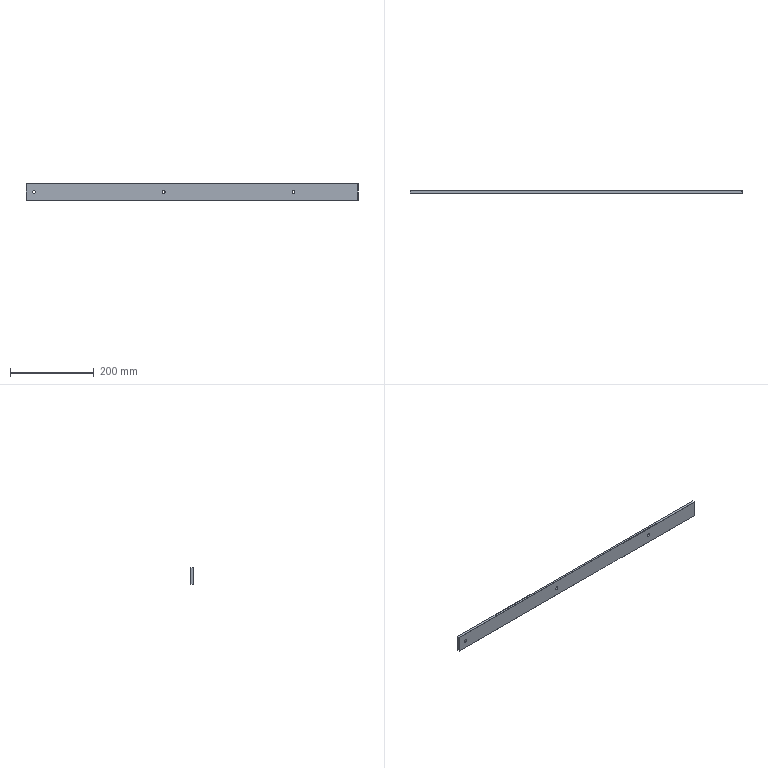Part | NX | 1 solid | 24 faces | box 793 x 6 x 40 mm | volume 189476 mm3 | plane 18 | cylinder 6 | commonest cylinder face diameters 7 x6
STEP:
#1=CARTESIAN_POINT('',(0.3,0.,-19.7));
#2=VERTEX_POINT('',#1);
#3=CARTESIAN_POINT('',(792.7,0.,-19.7));
#4=VERTEX_POINT('',#3);
#5=CARTESIAN_POINT('',(396.5,0.,-19.7));
#6=DIRECTION('',(1.,0.,0.));
#7=VECTOR('',#6,1000.);
#8=LINE('',#5,#7);
#9=EDGE_CURVE('',#2,#4,#8,.T.);
#10=ORIENTED_EDGE('',*,*,#9,.T.);
#11=CARTESIAN_POINT('',(792.7,0.,19.7));
#12=VERTEX_POINT('',#11);
#13=CARTESIAN_POINT('',(792.7,0.,0.));
#14=DIRECTION('',(0.,0.,1.));
#15=VECTOR('',#14,1000.);
#16=LINE('',#13,#15);
#17=EDGE_CURVE('',#4,#12,#16,.T.);
#18=ORIENTED_EDGE('',*,*,#17,.T.);
#19=CARTESIAN_POINT('',(0.3,0.,19.7));
#20=VERTEX_POINT('',#19);
#21=CARTESIAN_POINT('',(396.5,0.,19.7));
#22=DIRECTION('',(-1.,0.,0.));
#23=VECTOR('',#22,1000.);
#24=LINE('',#21,#23);
#25=EDGE_CURVE('',#12,#20,#24,.T.);
#26=ORIENTED_EDGE('',*,*,#25,.T.);
#27=CARTESIAN_POINT('',(0.3,0.,0.));
#28=DIRECTION('',(0.,0.,-1.));
#29=VECTOR('',#28,1000.);
#30=LINE('',#27,#29);
#31=EDGE_CURVE('',#20,#2,#30,.T.);
#32=ORIENTED_EDGE('',*,*,#31,.T.);
#33=EDGE_LOOP('',(#10,#18,#26,#32));
#34=FACE_BOUND('',#33,.T.);
#35=CARTESIAN_POINT('',(332.5,0.,0.));
#36=VERTEX_POINT('',#35);
#37=CARTESIAN_POINT('',(325.5,0.,0.));
#38=VERTEX_POINT('',#37);
#39=CARTESIAN_POINT('',(329.,0.,0.));
#40=DIRECTION('',(0.,-1.,0.));
#41=DIRECTION('',(-1.,0.,0.));
#42=AXIS2_PLACEMENT_3D('',#39,#40,#41);
#43=CIRCLE('',#42,3.5);
#44=EDGE_CURVE('',#36,#38,#43,.T.);
#45=ORIENTED_EDGE('',*,*,#44,.F.);
#46=CARTESIAN_POINT('',(329.,0.,0.));
#47=DIRECTION('',(0.,-1.,0.));
#48=DIRECTION('',(-1.,0.,0.));
#49=AXIS2_PLACEMENT_3D('',#46,#47,#48);
#50=CIRCLE('',#49,3.5);
#51=EDGE_CURVE('',#38,#36,#50,.T.);
#52=ORIENTED_EDGE('',*,*,#51,.F.);
#53=EDGE_LOOP('',(#45,#52));
#54=FACE_BOUND('',#53,.T.);
#55=CARTESIAN_POINT('',(642.5,0.,0.));
#56=VERTEX_POINT('',#55);
#57=CARTESIAN_POINT('',(635.5,0.,0.));
#58=VERTEX_POINT('',#57);
#59=CARTESIAN_POINT('',(639.,0.,0.));
#60=DIRECTION('',(0.,-1.,0.));
#61=DIRECTION('',(-1.,0.,0.));
#62=AXIS2_PLACEMENT_3D('',#59,#60,#61);
#63=CIRCLE('',#62,3.5);
#64=EDGE_CURVE('',#56,#58,#63,.T.);
#65=ORIENTED_EDGE('',*,*,#64,.F.);
#66=CARTESIAN_POINT('',(639.,0.,0.));
#67=DIRECTION('',(0.,-1.,0.));
#68=DIRECTION('',(-1.,0.,0.));
#69=AXIS2_PLACEMENT_3D('',#66,#67,#68);
#70=CIRCLE('',#69,3.5);
#71=EDGE_CURVE('',#58,#56,#70,.T.);
#72=ORIENTED_EDGE('',*,*,#71,.F.);
#73=EDGE_LOOP('',(#65,#72));
#74=FACE_BOUND('',#73,.T.);
#75=CARTESIAN_POINT('',(15.5,0.,0.));
#76=VERTEX_POINT('',#75);
#77=CARTESIAN_POINT('',(22.5,0.,0.));
#78=VERTEX_POINT('',#77);
#79=CARTESIAN_POINT('',(19.,0.,0.));
#80=DIRECTION('',(0.,-1.,0.));
#81=DIRECTION('',(-1.,0.,0.));
#82=AXIS2_PLACEMENT_3D('',#79,#80,#81);
#83=CIRCLE('',#82,3.5);
#84=EDGE_CURVE('',#76,#78,#83,.T.);
#85=ORIENTED_EDGE('',*,*,#84,.F.);
#86=CARTESIAN_POINT('',(19.,0.,0.));
#87=DIRECTION('',(0.,-1.,0.));
#88=DIRECTION('',(-1.,0.,0.));
#89=AXIS2_PLACEMENT_3D('',#86,#87,#88);
#90=CIRCLE('',#89,3.5);
#91=EDGE_CURVE('',#78,#76,#90,.T.);
#92=ORIENTED_EDGE('',*,*,#91,.F.);
#93=EDGE_LOOP('',(#85,#92));
#94=FACE_BOUND('',#93,.T.);
#95=CARTESIAN_POINT('',(0.,0.,0.));
#96=DIRECTION('',(0.,1.,0.));
#97=DIRECTION('',(1.,0.,0.));
#98=AXIS2_PLACEMENT_3D('',#95,#96,#97);
#99=PLANE('',#98);
#100=ADVANCED_FACE('',(#34,#54,#74,#94),#99,.F.);
#101=CARTESIAN_POINT('',(0.,5.7,-19.7));
#102=VERTEX_POINT('',#101);
#103=CARTESIAN_POINT('',(0.,0.3,-19.7));
#104=VERTEX_POINT('',#103);
#105=CARTESIAN_POINT('',(0.,3.,-19.7));
#106=DIRECTION('',(0.,-1.,0.));
#107=VECTOR('',#106,1000.);
#108=LINE('',#105,#107);
#109=EDGE_CURVE('',#102,#104,#108,.T.);
#110=ORIENTED_EDGE('',*,*,#109,.T.);
#111=CARTESIAN_POINT('',(0.,0.3,19.7));
#112=VERTEX_POINT('',#111);
#113=CARTESIAN_POINT('',(0.,0.3,0.));
#114=DIRECTION('',(0.,0.,-1.));
#115=VECTOR('',#114,1000.);
#116=LINE('',#113,#115);
#117=EDGE_CURVE('',#112,#104,#116,.T.);
#118=ORIENTED_EDGE('',*,*,#117,.F.);
#119=CARTESIAN_POINT('',(0.,5.7,19.7));
#120=VERTEX_POINT('',#119);
#121=CARTESIAN_POINT('',(0.,3.,19.7));
#122=DIRECTION('',(0.,-1.,0.));
#123=VECTOR('',#122,1000.);
#124=LINE('',#121,#123);
#125=EDGE_CURVE('',#120,#112,#124,.T.);
#126=ORIENTED_EDGE('',*,*,#125,.F.);
#127=CARTESIAN_POINT('',(0.,5.7,0.));
#128=DIRECTION('',(0.,0.,-1.));
#129=VECTOR('',#128,1000.);
#130=LINE('',#127,#129);
#131=EDGE_CURVE('',#120,#102,#130,.T.);
#132=ORIENTED_EDGE('',*,*,#131,.T.);
#133=EDGE_LOOP('',(#110,#118,#126,#132));
#134=FACE_BOUND('',#133,.T.);
#135=CARTESIAN_POINT('',(0.,0.,-20.));
#136=DIRECTION('',(-1.,0.,0.));
#137=DIRECTION('',(0.,0.,1.));
#138=AXIS2_PLACEMENT_3D('',#135,#136,#137);
#139=PLANE('',#138);
#140=ADVANCED_FACE('',(#134),#139,.T.);
#141=CARTESIAN_POINT('',(0.3,5.7,-20.));
#142=VERTEX_POINT('',#141);
#143=CARTESIAN_POINT('',(792.7,5.7,-20.));
#144=VERTEX_POINT('',#143);
#145=CARTESIAN_POINT('',(396.5,5.7,-20.));
#146=DIRECTION('',(1.,0.,0.));
#147=VECTOR('',#146,1000.);
#148=LINE('',#145,#147);
#149=EDGE_CURVE('',#142,#144,#148,.T.);
#150=ORIENTED_EDGE('',*,*,#149,.T.);
#151=CARTESIAN_POINT('',(792.7,0.3,-20.));
#152=VERTEX_POINT('',#151);
#153=CARTESIAN_POINT('',(792.7,3.,-20.));
#154=DIRECTION('',(0.,-1.,0.));
#155=VECTOR('',#154,1000.);
#156=LINE('',#153,#155);
#157=EDGE_CURVE('',#144,#152,#156,.T.);
#158=ORIENTED_EDGE('',*,*,#157,.T.);
#159=CARTESIAN_POINT('',(0.3,0.3,-20.));
#160=VERTEX_POINT('',#159);
#161=CARTESIAN_POINT('',(396.5,0.3,-20.));
#162=DIRECTION('',(1.,0.,0.));
#163=VECTOR('',#162,1000.);
#164=LINE('',#161,#163);
#165=EDGE_CURVE('',#160,#152,#164,.T.);
#166=ORIENTED_EDGE('',*,*,#165,.F.);
#167=CARTESIAN_POINT('',(0.3,3.,-20.));
#168=DIRECTION('',(0.,-1.,0.));
#169=VECTOR('',#168,1000.);
#170=LINE('',#167,#169);
#171=EDGE_CURVE('',#142,#160,#170,.T.);
#172=ORIENTED_EDGE('',*,*,#171,.F.);
#173=EDGE_LOOP('',(#150,#158,#166,#172));
#174=FACE_BOUND('',#173,.T.);
#175=CARTESIAN_POINT('',(793.,0.,-20.));
#176=DIRECTION('',(0.,0.,-1.));
#177=DIRECTION('',(0.,-1.,0.));
#178=AXIS2_PLACEMENT_3D('',#175,#176,#177);
#179=PLANE('',#178);
#180=ADVANCED_FACE('',(#174),#179,.T.);
#181=CARTESIAN_POINT('',(793.,5.7,-19.7));
#182=VERTEX_POINT('',#181);
#183=CARTESIAN_POINT('',(793.,5.7,19.7));
#184=VERTEX_POINT('',#183);
#185=CARTESIAN_POINT('',(793.,5.7,0.));
#186=DIRECTION('',(0.,0.,1.));
#187=VECTOR('',#186,1000.);
#188=LINE('',#185,#187);
#189=EDGE_CURVE('',#182,#184,#188,.T.);
#190=ORIENTED_EDGE('',*,*,#189,.T.);
#191=CARTESIAN_POINT('',(793.,0.3,19.7));
#192=VERTEX_POINT('',#191);
#193=CARTESIAN_POINT('',(793.,3.,19.7));
#194=DIRECTION('',(0.,-1.,0.));
#195=VECTOR('',#194,1000.);
#196=LINE('',#193,#195);
#197=EDGE_CURVE('',#184,#192,#196,.T.);
#198=ORIENTED_EDGE('',*,*,#197,.T.);
#199=CARTESIAN_POINT('',(793.,0.3,-19.7));
#200=VERTEX_POINT('',#199);
#201=CARTESIAN_POINT('',(793.,0.3,0.));
#202=DIRECTION('',(0.,0.,1.));
#203=VECTOR('',#202,1000.);
#204=LINE('',#201,#203);
#205=EDGE_CURVE('',#200,#192,#204,.T.);
#206=ORIENTED_EDGE('',*,*,#205,.F.);
#207=CARTESIAN_POINT('',(793.,3.,-19.7));
#208=DIRECTION('',(0.,-1.,0.));
#209=VECTOR('',#208,1000.);
#210=LINE('',#207,#209);
#211=EDGE_CURVE('',#182,#200,#210,.T.);
#212=ORIENTED_EDGE('',*,*,#211,.F.);
#213=EDGE_LOOP('',(#190,#198,#206,#212));
#214=FACE_BOUND('',#213,.T.);
#215=CARTESIAN_POINT('',(793.,0.,20.));
#216=DIRECTION('',(1.,0.,0.));
#217=DIRECTION('',(0.,1.,0.));
#218=AXIS2_PLACEMENT_3D('',#215,#216,#217);
#219=PLANE('',#218);
#220=ADVANCED_FACE('',(#214),#219,.T.);
#221=CARTESIAN_POINT('',(792.7,5.7,20.));
#222=VERTEX_POINT('',#221);
#223=CARTESIAN_POINT('',(0.3,5.7,20.));
#224=VERTEX_POINT('',#223);
#225=CARTESIAN_POINT('',(396.5,5.7,20.));
#226=DIRECTION('',(-1.,0.,0.));
#227=VECTOR('',#226,1000.);
#228=LINE('',#225,#227);
#229=EDGE_CURVE('',#222,#224,#228,.T.);
#230=ORIENTED_EDGE('',*,*,#229,.T.);
#231=CARTESIAN_POINT('',(0.3,0.3,20.));
#232=VERTEX_POINT('',#231);
#233=CARTESIAN_POINT('',(0.3,3.,20.));
#234=DIRECTION('',(0.,-1.,0.));
#235=VECTOR('',#234,1000.);
#236=LINE('',#233,#235);
#237=EDGE_CURVE('',#224,#232,#236,.T.);
#238=ORIENTED_EDGE('',*,*,#237,.T.);
#239=CARTESIAN_POINT('',(792.7,0.3,20.));
#240=VERTEX_POINT('',#239);
#241=CARTESIAN_POINT('',(396.5,0.3,20.));
#242=DIRECTION('',(-1.,0.,0.));
#243=VECTOR('',#242,1000.);
#244=LINE('',#241,#243);
#245=EDGE_CURVE('',#240,#232,#244,.T.);
#246=ORIENTED_EDGE('',*,*,#245,.F.);
#247=CARTESIAN_POINT('',(792.7,3.,20.));
#248=DIRECTION('',(0.,-1.,0.));
#249=VECTOR('',#248,1000.);
#250=LINE('',#247,#249);
#251=EDGE_CURVE('',#222,#240,#250,.T.);
#252=ORIENTED_EDGE('',*,*,#251,.F.);
#253=EDGE_LOOP('',(#230,#238,#246,#252));
#254=FACE_BOUND('',#253,.T.);
#255=CARTESIAN_POINT('',(0.,0.,20.));
#256=DIRECTION('',(0.,0.,1.));
#257=DIRECTION('',(1.,0.,0.));
#258=AXIS2_PLACEMENT_3D('',#255,#256,#257);
#259=PLANE('',#258);
#260=ADVANCED_FACE('',(#254),#259,.T.);
#261=CARTESIAN_POINT('',(0.3,6.,19.7));
#262=VERTEX_POINT('',#261);
#263=CARTESIAN_POINT('',(0.3,6.,-19.7));
#264=VERTEX_POINT('',#263);
#265=CARTESIAN_POINT('',(0.3,6.,0.));
#266=DIRECTION('',(0.,0.,-1.));
#267=VECTOR('',#266,1000.);
#268=LINE('',#265,#267);
#269=EDGE_CURVE('',#262,#264,#268,.T.);
#270=ORIENTED_EDGE('',*,*,#269,.F.);
#271=CARTESIAN_POINT('',(792.7,6.,19.7));
#272=VERTEX_POINT('',#271);
#273=CARTESIAN_POINT('',(396.5,6.,19.7));
#274=DIRECTION('',(-1.,0.,0.));
#275=VECTOR('',#274,1000.);
#276=LINE('',#273,#275);
#277=EDGE_CURVE('',#272,#262,#276,.T.);
#278=ORIENTED_EDGE('',*,*,#277,.F.);
#279=CARTESIAN_POINT('',(792.7,6.,-19.7));
#280=VERTEX_POINT('',#279);
#281=CARTESIAN_POINT('',(792.7,6.,0.));
#282=DIRECTION('',(0.,0.,1.));
#283=VECTOR('',#282,1000.);
#284=LINE('',#281,#283);
#285=EDGE_CURVE('',#280,#272,#284,.T.);
#286=ORIENTED_EDGE('',*,*,#285,.F.);
#287=CARTESIAN_POINT('',(396.5,6.,-19.7));
#288=DIRECTION('',(1.,0.,0.));
#289=VECTOR('',#288,1000.);
#290=LINE('',#287,#289);
#291=EDGE_CURVE('',#264,#280,#290,.T.);
#292=ORIENTED_EDGE('',*,*,#291,.F.);
#293=EDGE_LOOP('',(#270,#278,#286,#292));
#294=FACE_BOUND('',#293,.T.);
#295=CARTESIAN_POINT('',(332.5,6.,0.));
#296=VERTEX_POINT('',#295);
#297=CARTESIAN_POINT('',(325.5,6.,0.));
#298=VERTEX_POINT('',#297);
#299=CARTESIAN_POINT('',(329.,6.,0.));
#300=DIRECTION('',(0.,1.,0.));
#301=DIRECTION('',(1.,0.,0.));
#302=AXIS2_PLACEMENT_3D('',#299,#300,#301);
#303=CIRCLE('',#302,3.5);
#304=EDGE_CURVE('',#296,#298,#303,.T.);
#305=ORIENTED_EDGE('',*,*,#304,.F.);
#306=CARTESIAN_POINT('',(329.,6.,0.));
#307=DIRECTION('',(0.,1.,0.));
#308=DIRECTION('',(1.,0.,0.));
#309=AXIS2_PLACEMENT_3D('',#306,#307,#308);
#310=CIRCLE('',#309,3.5);
#311=EDGE_CURVE('',#298,#296,#310,.T.);
#312=ORIENTED_EDGE('',*,*,#311,.F.);
#313=EDGE_LOOP('',(#305,#312));
#314=FACE_BOUND('',#313,.T.);
#315=CARTESIAN_POINT('',(635.5,6.,0.));
#316=VERTEX_POINT('',#315);
#317=CARTESIAN_POINT('',(642.5,6.,0.));
#318=VERTEX_POINT('',#317);
#319=CARTESIAN_POINT('',(639.,6.,0.));
#320=DIRECTION('',(0.,1.,0.));
#321=DIRECTION('',(1.,0.,0.));
#322=AXIS2_PLACEMENT_3D('',#319,#320,#321);
#323=CIRCLE('',#322,3.5);
#324=EDGE_CURVE('',#316,#318,#323,.T.);
#325=ORIENTED_EDGE('',*,*,#324,.F.);
#326=CARTESIAN_POINT('',(639.,6.,0.));
#327=DIRECTION('',(0.,1.,0.));
#328=DIRECTION('',(1.,0.,0.));
#329=AXIS2_PLACEMENT_3D('',#326,#327,#328);
#330=CIRCLE('',#329,3.5);
#331=EDGE_CURVE('',#318,#316,#330,.T.);
#332=ORIENTED_EDGE('',*,*,#331,.F.);
#333=EDGE_LOOP('',(#325,#332));
#334=FACE_BOUND('',#333,.T.);
#335=CARTESIAN_POINT('',(22.5,6.,0.));
#336=VERTEX_POINT('',#335);
#337=CARTESIAN_POINT('',(15.5,6.,0.));
#338=VERTEX_POINT('',#337);
#339=CARTESIAN_POINT('',(19.,6.,0.));
#340=DIRECTION('',(0.,1.,0.));
#341=DIRECTION('',(1.,0.,0.));
#342=AXIS2_PLACEMENT_3D('',#339,#340,#341);
#343=CIRCLE('',#342,3.5);
#344=EDGE_CURVE('',#336,#338,#343,.T.);
#345=ORIENTED_EDGE('',*,*,#344,.F.);
#346=CARTESIAN_POINT('',(19.,6.,0.));
#347=DIRECTION('',(0.,1.,0.));
#348=DIRECTION('',(1.,0.,0.));
#349=AXIS2_PLACEMENT_3D('',#346,#347,#348);
#350=CIRCLE('',#349,3.5);
#351=EDGE_CURVE('',#338,#336,#350,.T.);
#352=ORIENTED_EDGE('',*,*,#351,.F.);
#353=EDGE_LOOP('',(#345,#352));
#354=FACE_BOUND('',#353,.T.);
#355=CARTESIAN_POINT('',(0.,6.,0.));
#356=DIRECTION('',(0.,1.,0.));
#357=DIRECTION('',(1.,0.,0.));
#358=AXIS2_PLACEMENT_3D('',#355,#356,#357);
#359=PLANE('',#358);
#360=ADVANCED_FACE('',(#294,#314,#334,#354),#359,.T.);
#361=ORIENTED_EDGE('',*,*,#84,.T.);
#362=CARTESIAN_POINT('',(22.5,6.,0.));
#363=DIRECTION('',(0.,-1.,0.));
#364=VECTOR('',#363,1000.);
#365=LINE('',#362,#364);
#366=EDGE_CURVE('',#336,#78,#365,.T.);
#367=ORIENTED_EDGE('',*,*,#366,.F.);
#368=ORIENTED_EDGE('',*,*,#344,.T.);
#369=CARTESIAN_POINT('',(15.5,6.,0.));
#370=DIRECTION('',(0.,-1.,0.));
#371=VECTOR('',#370,1000.);
#372=LINE('',#369,#371);
#373=EDGE_CURVE('',#338,#76,#372,.T.);
#374=ORIENTED_EDGE('',*,*,#373,.T.);
#375=EDGE_LOOP('',(#361,#367,#368,#374));
#376=FACE_BOUND('',#375,.T.);
#377=CARTESIAN_POINT('',(19.,6.,0.));
#378=DIRECTION('',(0.,-1.,0.));
#379=DIRECTION('',(1.,0.,0.));
#380=AXIS2_PLACEMENT_3D('',#377,#378,#379);
#381=CYLINDRICAL_SURFACE('',#380,3.5);
#382=ADVANCED_FACE('',(#376),#381,.F.);
#383=ORIENTED_EDGE('',*,*,#64,.T.);
#384=CARTESIAN_POINT('',(635.5,6.,0.));
#385=DIRECTION('',(0.,-1.,0.));
#386=VECTOR('',#385,1000.);
#387=LINE('',#384,#386);
#388=EDGE_CURVE('',#316,#58,#387,.T.);
#389=ORIENTED_EDGE('',*,*,#388,.F.);
#390=ORIENTED_EDGE('',*,*,#324,.T.);
#391=CARTESIAN_POINT('',(642.5,6.,0.));
#392=DIRECTION('',(0.,-1.,0.));
#393=VECTOR('',#392,1000.);
#394=LINE('',#391,#393);
#395=EDGE_CURVE('',#318,#56,#394,.T.);
#396=ORIENTED_EDGE('',*,*,#395,.T.);
#397=EDGE_LOOP('',(#383,#389,#390,#396));
#398=FACE_BOUND('',#397,.T.);
#399=CARTESIAN_POINT('',(639.,6.,0.));
#400=DIRECTION('',(0.,-1.,0.));
#401=DIRECTION('',(1.,0.,0.));
#402=AXIS2_PLACEMENT_3D('',#399,#400,#401);
#403=CYLINDRICAL_SURFACE('',#402,3.5);
#404=ADVANCED_FACE('',(#398),#403,.F.);
#405=ORIENTED_EDGE('',*,*,#304,.T.);
#406=CARTESIAN_POINT('',(325.5,6.,0.));
#407=DIRECTION('',(0.,-1.,0.));
#408=VECTOR('',#407,1000.);
#409=LINE('',#406,#408);
#410=EDGE_CURVE('',#38,#298,#409,.F.);
#411=ORIENTED_EDGE('',*,*,#410,.F.);
#412=ORIENTED_EDGE('',*,*,#51,.T.);
#413=CARTESIAN_POINT('',(332.5,6.,0.));
#414=DIRECTION('',(0.,-1.,0.));
#415=VECTOR('',#414,1000.);
#416=LINE('',#413,#415);
#417=EDGE_CURVE('',#36,#296,#416,.F.);
#418=ORIENTED_EDGE('',*,*,#417,.T.);
#419=EDGE_LOOP('',(#405,#411,#412,#418));
#420=FACE_BOUND('',#419,.T.);
#421=CARTESIAN_POINT('',(329.,6.,0.));
#422=DIRECTION('',(0.,-1.,0.));
#423=DIRECTION('',(1.,0.,0.));
#424=AXIS2_PLACEMENT_3D('',#421,#422,#423);
#425=CYLINDRICAL_SURFACE('',#424,3.5);
#426=ADVANCED_FACE('',(#420),#425,.F.);
#427=ORIENTED_EDGE('',*,*,#131,.F.);
#428=CARTESIAN_POINT('',(0.15,5.85,19.85));
#429=VERTEX_POINT('',#428);
#430=CARTESIAN_POINT('',(0.,5.7,19.7));
#431=DIRECTION('',(-0.5774,-0.5774,-0.5774));
#432=VECTOR('',#431,1000.);
#433=LINE('',#430,#432);
#434=EDGE_CURVE('',#429,#120,#433,.T.);
#435=ORIENTED_EDGE('',*,*,#434,.F.);
#436=CARTESIAN_POINT('',(20.,25.7,0.));
#437=DIRECTION('',(0.5774,0.5774,-0.5774));
#438=VECTOR('',#437,1000.);
#439=LINE('',#436,#438);
#440=EDGE_CURVE('',#429,#262,#439,.T.);
#441=ORIENTED_EDGE('',*,*,#440,.T.);
#442=ORIENTED_EDGE('',*,*,#269,.T.);
#443=CARTESIAN_POINT('',(0.15,5.85,-19.85));
#444=VERTEX_POINT('',#443);
#445=CARTESIAN_POINT('',(20.,25.7,0.));
#446=DIRECTION('',(-0.5774,-0.5774,-0.5774));
#447=VECTOR('',#446,1000.);
#448=LINE('',#445,#447);
#449=EDGE_CURVE('',#264,#444,#448,.T.);
#450=ORIENTED_EDGE('',*,*,#449,.T.);
#451=CARTESIAN_POINT('',(-19.7,-14.,0.));
#452=DIRECTION('',(-0.5774,-0.5774,0.5774));
#453=VECTOR('',#452,1000.);
#454=LINE('',#451,#453);
#455=EDGE_CURVE('',#444,#102,#454,.T.);
#456=ORIENTED_EDGE('',*,*,#455,.T.);
#457=EDGE_LOOP('',(#427,#435,#441,#442,#450,#456));
#458=FACE_BOUND('',#457,.T.);
#459=CARTESIAN_POINT('',(0.15,5.85,0.));
#460=DIRECTION('',(-0.7071,0.7071,0.));
#461=DIRECTION('',(0.,0.,1.));
#462=AXIS2_PLACEMENT_3D('',#459,#460,#461);
#463=PLANE('',#462);
#464=ADVANCED_FACE('',(#458),#463,.T.);
#465=ORIENTED_EDGE('',*,*,#31,.F.);
#466=CARTESIAN_POINT('',(0.15,0.15,19.85));
#467=VERTEX_POINT('',#466);
#468=CARTESIAN_POINT('',(20.,-19.7,0.));
#469=DIRECTION('',(-0.5774,0.5774,0.5774));
#470=VECTOR('',#469,1000.);
#471=LINE('',#468,#470);
#472=EDGE_CURVE('',#20,#467,#471,.T.);
#473=ORIENTED_EDGE('',*,*,#472,.T.);
#474=CARTESIAN_POINT('',(0.3,0.,20.));
#475=DIRECTION('',(0.5774,-0.5774,0.5774));
#476=VECTOR('',#475,1000.);
#477=LINE('',#474,#476);
#478=EDGE_CURVE('',#112,#467,#477,.T.);
#479=ORIENTED_EDGE('',*,*,#478,.F.);
#480=ORIENTED_EDGE('',*,*,#117,.T.);
#481=CARTESIAN_POINT('',(0.15,0.15,-19.85));
#482=VERTEX_POINT('',#481);
#483=CARTESIAN_POINT('',(-19.7,20.,0.));
#484=DIRECTION('',(0.5774,-0.5774,-0.5774));
#485=VECTOR('',#484,1000.);
#486=LINE('',#483,#485);
#487=EDGE_CURVE('',#104,#482,#486,.T.);
#488=ORIENTED_EDGE('',*,*,#487,.T.);
#489=CARTESIAN_POINT('',(20.,-19.7,0.));
#490=DIRECTION('',(0.5774,-0.5774,0.5774));
#491=VECTOR('',#490,1000.);
#492=LINE('',#489,#491);
#493=EDGE_CURVE('',#482,#2,#492,.T.);
#494=ORIENTED_EDGE('',*,*,#493,.T.);
#495=EDGE_LOOP('',(#465,#473,#479,#480,#488,#494));
#496=FACE_BOUND('',#495,.T.);
#497=CARTESIAN_POINT('',(0.15,0.15,0.));
#498=DIRECTION('',(-0.7071,-0.7071,0.));
#499=DIRECTION('',(-0.7071,0.7071,0.));
#500=AXIS2_PLACEMENT_3D('',#497,#498,#499);
#501=PLANE('',#500);
#502=ADVANCED_FACE('',(#496),#501,.T.);
#503=ORIENTED_EDGE('',*,*,#125,.T.);
#504=ORIENTED_EDGE('',*,*,#478,.T.);
#505=CARTESIAN_POINT('',(0.,0.,19.7));
#506=DIRECTION('',(-0.5774,-0.5774,-0.5774));
#507=VECTOR('',#506,1000.);
#508=LINE('',#505,#507);
#509=EDGE_CURVE('',#232,#467,#508,.T.);
#510=ORIENTED_EDGE('',*,*,#509,.F.);
#511=ORIENTED_EDGE('',*,*,#237,.F.);
#512=CARTESIAN_POINT('',(0.,6.,19.7));
#513=DIRECTION('',(0.5774,-0.5774,0.5774));
#514=VECTOR('',#513,1000.);
#515=LINE('',#512,#514);
#516=EDGE_CURVE('',#429,#224,#515,.T.);
#517=ORIENTED_EDGE('',*,*,#516,.F.);
#518=ORIENTED_EDGE('',*,*,#434,.T.);
#519=EDGE_LOOP('',(#503,#504,#510,#511,#517,#518));
#520=FACE_BOUND('',#519,.T.);
#521=CARTESIAN_POINT('',(0.15,3.,19.85));
#522=DIRECTION('',(0.7071,0.,-0.7071));
#523=DIRECTION('',(0.,-1.,0.));
#524=AXIS2_PLACEMENT_3D('',#521,#522,#523);
#525=PLANE('',#524);
#526=ADVANCED_FACE('',(#520),#525,.F.);
#527=ORIENTED_EDGE('',*,*,#229,.F.);
#528=CARTESIAN_POINT('',(792.85,5.85,19.85));
#529=VERTEX_POINT('',#528);
#530=CARTESIAN_POINT('',(812.7,25.7,0.));
#531=DIRECTION('',(0.5774,0.5774,-0.5774));
#532=VECTOR('',#531,1000.);
#533=LINE('',#530,#532);
#534=EDGE_CURVE('',#222,#529,#533,.T.);
#535=ORIENTED_EDGE('',*,*,#534,.T.);
#536=CARTESIAN_POINT('',(773.,25.7,0.));
#537=DIRECTION('',(-0.5774,0.5774,-0.5774));
#538=VECTOR('',#537,1000.);
#539=LINE('',#536,#538);
#540=EDGE_CURVE('',#529,#272,#539,.T.);
#541=ORIENTED_EDGE('',*,*,#540,.T.);
#542=ORIENTED_EDGE('',*,*,#277,.T.);
#543=ORIENTED_EDGE('',*,*,#440,.F.);
#544=ORIENTED_EDGE('',*,*,#516,.T.);
#545=EDGE_LOOP('',(#527,#535,#541,#542,#543,#544));
#546=FACE_BOUND('',#545,.T.);
#547=CARTESIAN_POINT('',(396.5,5.85,19.85));
#548=DIRECTION('',(0.,0.7071,0.7071));
#549=DIRECTION('',(1.,0.,0.));
#550=AXIS2_PLACEMENT_3D('',#547,#548,#549);
#551=PLANE('',#550);
#552=ADVANCED_FACE('',(#546),#551,.T.);
#553=ORIENTED_EDGE('',*,*,#25,.F.);
#554=CARTESIAN_POINT('',(792.85,0.15,19.85));
#555=VERTEX_POINT('',#554);
#556=CARTESIAN_POINT('',(773.,-19.7,0.));
#557=DIRECTION('',(0.5774,0.5774,0.5774));
#558=VECTOR('',#557,1000.);
#559=LINE('',#556,#558);
#560=EDGE_CURVE('',#12,#555,#559,.T.);
#561=ORIENTED_EDGE('',*,*,#560,.T.);
#562=CARTESIAN_POINT('',(812.7,-19.7,0.));
#563=DIRECTION('',(-0.5774,0.5774,0.5774));
#564=VECTOR('',#563,1000.);
#565=LINE('',#562,#564);
#566=EDGE_CURVE('',#555,#240,#565,.T.);
#567=ORIENTED_EDGE('',*,*,#566,.T.);
#568=ORIENTED_EDGE('',*,*,#245,.T.);
#569=ORIENTED_EDGE('',*,*,#509,.T.);
#570=ORIENTED_EDGE('',*,*,#472,.F.);
#571=EDGE_LOOP('',(#553,#561,#567,#568,#569,#570));
#572=FACE_BOUND('',#571,.T.);
#573=CARTESIAN_POINT('',(396.5,0.15,19.85));
#574=DIRECTION('',(0.,-0.7071,0.7071));
#575=DIRECTION('',(-1.,0.,0.));
#576=AXIS2_PLACEMENT_3D('',#573,#574,#575);
#577=PLANE('',#576);
#578=ADVANCED_FACE('',(#572),#577,.T.);
#579=ORIENTED_EDGE('',*,*,#197,.F.);
#580=CARTESIAN_POINT('',(812.7,-14.,0.));
#581=DIRECTION('',(-0.5774,0.5774,0.5774));
#582=VECTOR('',#581,1000.);
#583=LINE('',#580,#582);
#584=EDGE_CURVE('',#184,#529,#583,.T.);
#585=ORIENTED_EDGE('',*,*,#584,.T.);
#586=ORIENTED_EDGE('',*,*,#534,.F.);
#587=ORIENTED_EDGE('',*,*,#251,.T.);
#588=ORIENTED_EDGE('',*,*,#566,.F.);
#589=CARTESIAN_POINT('',(812.7,20.,0.));
#590=DIRECTION('',(0.5774,0.5774,-0.5774));
#591=VECTOR('',#590,1000.);
#592=LINE('',#589,#591);
#593=EDGE_CURVE('',#555,#192,#592,.T.);
#594=ORIENTED_EDGE('',*,*,#593,.T.);
#595=EDGE_LOOP('',(#579,#585,#586,#587,#588,#594));
#596=FACE_BOUND('',#595,.T.);
#597=CARTESIAN_POINT('',(792.85,3.,19.85));
#598=DIRECTION('',(0.7071,0.,0.7071));
#599=DIRECTION('',(0.,-1.,0.));
#600=AXIS2_PLACEMENT_3D('',#597,#598,#599);
#601=PLANE('',#600);
#602=ADVANCED_FACE('',(#596),#601,.T.);
#603=ORIENTED_EDGE('',*,*,#189,.F.);
#604=CARTESIAN_POINT('',(792.85,5.85,-19.85));
#605=VERTEX_POINT('',#604);
#606=CARTESIAN_POINT('',(798.7,0.,-14.));
#607=DIRECTION('',(-0.5774,0.5774,-0.5774));
#608=VECTOR('',#607,1000.);
#609=LINE('',#606,#608);
#610=EDGE_CURVE('',#182,#605,#609,.T.);
#611=ORIENTED_EDGE('',*,*,#610,.T.);
#612=CARTESIAN_POINT('',(773.,25.7,0.));
#613=DIRECTION('',(-0.5774,0.5774,0.5774));
#614=VECTOR('',#613,1000.);
#615=LINE('',#612,#614);
#616=EDGE_CURVE('',#605,#280,#615,.T.);
#617=ORIENTED_EDGE('',*,*,#616,.T.);
#618=ORIENTED_EDGE('',*,*,#285,.T.);
#619=ORIENTED_EDGE('',*,*,#540,.F.);
#620=ORIENTED_EDGE('',*,*,#584,.F.);
#621=EDGE_LOOP('',(#603,#611,#617,#618,#619,#620));
#622=FACE_BOUND('',#621,.T.);
#623=CARTESIAN_POINT('',(792.85,5.85,0.));
#624=DIRECTION('',(0.7071,0.7071,0.));
#625=DIRECTION('',(0.,0.,-1.));
#626=AXIS2_PLACEMENT_3D('',#623,#624,#625);
#627=PLANE('',#626);
#628=ADVANCED_FACE('',(#622),#627,.T.);
#629=ORIENTED_EDGE('',*,*,#17,.F.);
#630=CARTESIAN_POINT('',(792.85,0.15,-19.85));
#631=VERTEX_POINT('',#630);
#632=CARTESIAN_POINT('',(773.,-19.7,0.));
#633=DIRECTION('',(0.5774,0.5774,-0.5774));
#634=VECTOR('',#633,1000.);
#635=LINE('',#632,#634);
#636=EDGE_CURVE('',#4,#631,#635,.T.);
#637=ORIENTED_EDGE('',*,*,#636,.T.);
#638=CARTESIAN_POINT('',(792.7,0.,-20.));
#639=DIRECTION('',(0.5774,0.5774,0.5774));
#640=VECTOR('',#639,1000.);
#641=LINE('',#638,#640);
#642=EDGE_CURVE('',#631,#200,#641,.T.);
#643=ORIENTED_EDGE('',*,*,#642,.T.);
#644=ORIENTED_EDGE('',*,*,#205,.T.);
#645=ORIENTED_EDGE('',*,*,#593,.F.);
#646=ORIENTED_EDGE('',*,*,#560,.F.);
#647=EDGE_LOOP('',(#629,#637,#643,#644,#645,#646));
#648=FACE_BOUND('',#647,.T.);
#649=CARTESIAN_POINT('',(792.85,0.15,0.));
#650=DIRECTION('',(0.7071,-0.7071,0.));
#651=DIRECTION('',(0.,0.,-1.));
#652=AXIS2_PLACEMENT_3D('',#649,#650,#651);
#653=PLANE('',#652);
#654=ADVANCED_FACE('',(#648),#653,.T.);
#655=ORIENTED_EDGE('',*,*,#157,.F.);
#656=CARTESIAN_POINT('',(812.7,25.7,0.));
#657=DIRECTION('',(0.5774,0.5774,0.5774));
#658=VECTOR('',#657,1000.);
#659=LINE('',#656,#658);
#660=EDGE_CURVE('',#144,#605,#659,.T.);
#661=ORIENTED_EDGE('',*,*,#660,.T.);
#662=ORIENTED_EDGE('',*,*,#610,.F.);
#663=ORIENTED_EDGE('',*,*,#211,.T.);
#664=ORIENTED_EDGE('',*,*,#642,.F.);
#665=CARTESIAN_POINT('',(812.7,-19.7,0.));
#666=DIRECTION('',(-0.5774,0.5774,-0.5774));
#667=VECTOR('',#666,1000.);
#668=LINE('',#665,#667);
#669=EDGE_CURVE('',#631,#152,#668,.T.);
#670=ORIENTED_EDGE('',*,*,#669,.T.);
#671=EDGE_LOOP('',(#655,#661,#662,#663,#664,#670));
#672=FACE_BOUND('',#671,.T.);
#673=CARTESIAN_POINT('',(792.85,3.,-19.85));
#674=DIRECTION('',(0.7071,0.,-0.7071));
#675=DIRECTION('',(0.,-1.,0.));
#676=AXIS2_PLACEMENT_3D('',#673,#674,#675);
#677=PLANE('',#676);
#678=ADVANCED_FACE('',(#672),#677,.T.);
#679=ORIENTED_EDGE('',*,*,#9,.F.);
#680=ORIENTED_EDGE('',*,*,#493,.F.);
#681=CARTESIAN_POINT('',(-19.7,-19.7,0.));
#682=DIRECTION('',(0.5774,0.5774,-0.5774));
#683=VECTOR('',#682,1000.);
#684=LINE('',#681,#683);
#685=EDGE_CURVE('',#482,#160,#684,.T.);
#686=ORIENTED_EDGE('',*,*,#685,.T.);
#687=ORIENTED_EDGE('',*,*,#165,.T.);
#688=ORIENTED_EDGE('',*,*,#669,.F.);
#689=ORIENTED_EDGE('',*,*,#636,.F.);
#690=EDGE_LOOP('',(#679,#680,#686,#687,#688,#689));
#691=FACE_BOUND('',#690,.T.);
#692=CARTESIAN_POINT('',(396.5,0.15,-19.85));
#693=DIRECTION('',(0.,-0.7071,-0.7071));
#694=DIRECTION('',(0.,0.7071,-0.7071));
#695=AXIS2_PLACEMENT_3D('',#692,#693,#694);
#696=PLANE('',#695);
#697=ADVANCED_FACE('',(#691),#696,.T.);
#698=ORIENTED_EDGE('',*,*,#149,.F.);
#699=CARTESIAN_POINT('',(-19.7,25.7,0.));
#700=DIRECTION('',(-0.5774,0.5774,0.5774));
#701=VECTOR('',#700,1000.);
#702=LINE('',#699,#701);
#703=EDGE_CURVE('',#142,#444,#702,.T.);
#704=ORIENTED_EDGE('',*,*,#703,.T.);
#705=ORIENTED_EDGE('',*,*,#449,.F.);
#706=ORIENTED_EDGE('',*,*,#291,.T.);
#707=ORIENTED_EDGE('',*,*,#616,.F.);
#708=ORIENTED_EDGE('',*,*,#660,.F.);
#709=EDGE_LOOP('',(#698,#704,#705,#706,#707,#708));
#710=FACE_BOUND('',#709,.T.);
#711=CARTESIAN_POINT('',(396.5,5.85,-19.85));
#712=DIRECTION('',(0.,0.7071,-0.7071));
#713=DIRECTION('',(-1.,0.,0.));
#714=AXIS2_PLACEMENT_3D('',#711,#712,#713);
#715=PLANE('',#714);
#716=ADVANCED_FACE('',(#710),#715,.T.);
#717=ORIENTED_EDGE('',*,*,#109,.F.);
#718=ORIENTED_EDGE('',*,*,#455,.F.);
#719=ORIENTED_EDGE('',*,*,#703,.F.);
#720=ORIENTED_EDGE('',*,*,#171,.T.);
#721=ORIENTED_EDGE('',*,*,#685,.F.);
#722=ORIENTED_EDGE('',*,*,#487,.F.);
#723=EDGE_LOOP('',(#717,#718,#719,#720,#721,#722));
#724=FACE_BOUND('',#723,.T.);
#725=CARTESIAN_POINT('',(0.15,3.,-19.85));
#726=DIRECTION('',(-0.7071,0.,-0.7071));
#727=DIRECTION('',(-0.7071,0.,0.7071));
#728=AXIS2_PLACEMENT_3D('',#725,#726,#727);
#729=PLANE('',#728);
#730=ADVANCED_FACE('',(#724),#729,.T.);
#731=ORIENTED_EDGE('',*,*,#44,.T.);
#732=ORIENTED_EDGE('',*,*,#410,.T.);
#733=ORIENTED_EDGE('',*,*,#311,.T.);
#734=ORIENTED_EDGE('',*,*,#417,.F.);
#735=EDGE_LOOP('',(#731,#732,#733,#734));
#736=FACE_BOUND('',#735,.T.);
#737=CARTESIAN_POINT('',(329.,6.,0.));
#738=DIRECTION('',(0.,-1.,0.));
#739=DIRECTION('',(1.,0.,0.));
#740=AXIS2_PLACEMENT_3D('',#737,#738,#739);
#741=CYLINDRICAL_SURFACE('',#740,3.5);
#742=ADVANCED_FACE('',(#736),#741,.F.);
#743=ORIENTED_EDGE('',*,*,#366,.T.);
#744=ORIENTED_EDGE('',*,*,#91,.T.);
#745=ORIENTED_EDGE('',*,*,#373,.F.);
#746=ORIENTED_EDGE('',*,*,#351,.T.);
#747=EDGE_LOOP('',(#743,#744,#745,#746));
#748=FACE_BOUND('',#747,.T.);
#749=CARTESIAN_POINT('',(19.,6.,0.));
#750=DIRECTION('',(0.,-1.,0.));
#751=DIRECTION('',(1.,0.,0.));
#752=AXIS2_PLACEMENT_3D('',#749,#750,#751);
#753=CYLINDRICAL_SURFACE('',#752,3.5);
#754=ADVANCED_FACE('',(#748),#753,.F.);
#755=ORIENTED_EDGE('',*,*,#395,.F.);
#756=ORIENTED_EDGE('',*,*,#331,.T.);
#757=ORIENTED_EDGE('',*,*,#388,.T.);
#758=ORIENTED_EDGE('',*,*,#71,.T.);
#759=EDGE_LOOP('',(#755,#756,#757,#758));
#760=FACE_BOUND('',#759,.T.);
#761=CARTESIAN_POINT('',(639.,6.,0.));
#762=DIRECTION('',(0.,-1.,0.));
#763=DIRECTION('',(1.,0.,0.));
#764=AXIS2_PLACEMENT_3D('',#761,#762,#763);
#765=CYLINDRICAL_SURFACE('',#764,3.5);
#766=ADVANCED_FACE('',(#760),#765,.F.);
#767=CLOSED_SHELL('',(#100,#140,#180,#220,#260,#360,#382,#404,#426,#464,#502,#526,#552,#578,#602,#628,#654,#678,#697,#716,#730,#742,#754,#766));
#768=MANIFOLD_SOLID_BREP('',#767);
#769=(LENGTH_UNIT()NAMED_UNIT(*)SI_UNIT(.MILLI.,.METRE.));
#770=UNCERTAINTY_MEASURE_WITH_UNIT(LENGTH_MEASURE(0.00001),#769,'','');
#771=(NAMED_UNIT(*)PLANE_ANGLE_UNIT()SI_UNIT($,.RADIAN.));
#772=(NAMED_UNIT(*)SI_UNIT($,.STERADIAN.)SOLID_ANGLE_UNIT());
#773=(GEOMETRIC_REPRESENTATION_CONTEXT(3)GLOBAL_UNCERTAINTY_ASSIGNED_CONTEXT((#770))GLOBAL_UNIT_ASSIGNED_CONTEXT((#769,#771,#772))REPRESENTATION_CONTEXT('',''));
#774=ADVANCED_BREP_SHAPE_REPRESENTATION('',(#768),#773);